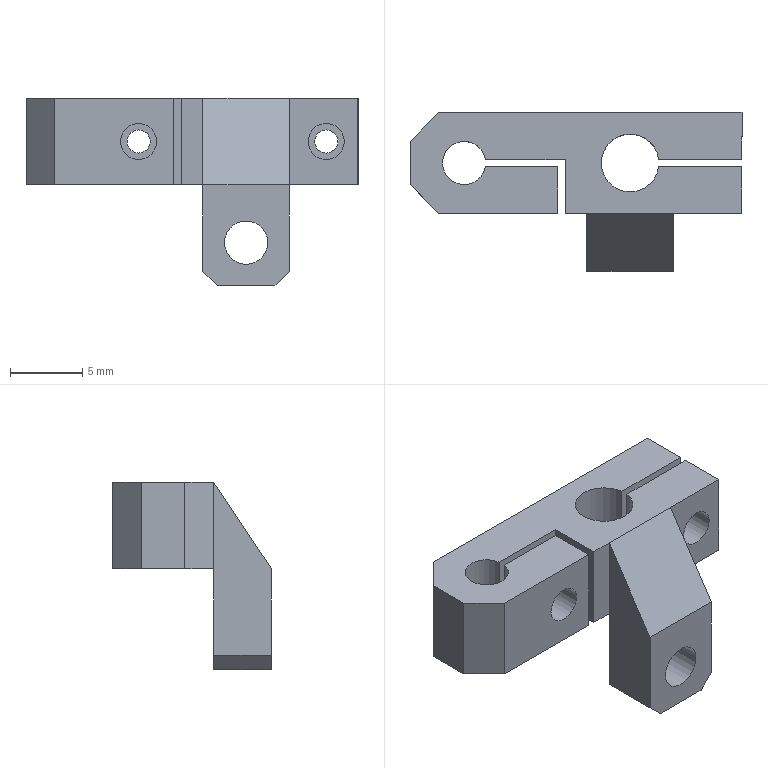Part | SolidWorks | features ICE 9, Chamfer 3, Extrusion 1, HoleWzd 1 | 1 solid | 39 faces | box 23 x 11 x 13 mm | volume 943.404 mm3 | plane 25 | cylinder 14 | commonest cylinder face diameters 1.6 x4 2.5 x4 3 x4 4 x2
STEP:
#1=CARTESIAN_POINT('',(-0.7,0.25,9.2));
#2=VERTEX_POINT('',#1);
#3=CARTESIAN_POINT('',(-0.7,0.25,10.8));
#4=VERTEX_POINT('',#3);
#5=CARTESIAN_POINT('',(-0.7,0.25,10.));
#6=DIRECTION('',(0.,1.,0.));
#7=DIRECTION('',(-1.,0.,0.));
#8=AXIS2_PLACEMENT_3D('',#5,#6,#7);
#9=CIRCLE('',#8,0.8);
#10=EDGE_CURVE('',#2,#4,#9,.T.);
#11=ORIENTED_EDGE('',*,*,#10,.F.);
#12=CARTESIAN_POINT('',(-0.7,3.5,9.2));
#13=VERTEX_POINT('',#12);
#14=CARTESIAN_POINT('',(-0.7,3.5,9.2));
#15=DIRECTION('',(0.,1.,0.));
#16=VECTOR('',#15,1000.);
#17=LINE('',#14,#16);
#18=EDGE_CURVE('',#2,#13,#17,.T.);
#19=ORIENTED_EDGE('',*,*,#18,.T.);
#20=CARTESIAN_POINT('',(-0.7,3.5,10.8));
#21=VERTEX_POINT('',#20);
#22=CARTESIAN_POINT('',(-0.7,3.5,10.));
#23=DIRECTION('',(0.,1.,0.));
#24=DIRECTION('',(0.,0.,1.));
#25=AXIS2_PLACEMENT_3D('',#22,#23,#24);
#26=CIRCLE('',#25,0.8);
#27=EDGE_CURVE('',#13,#21,#26,.T.);
#28=ORIENTED_EDGE('',*,*,#27,.T.);
#29=CARTESIAN_POINT('',(-0.7,3.5,10.8));
#30=DIRECTION('',(0.,1.,0.));
#31=VECTOR('',#30,1000.);
#32=LINE('',#29,#31);
#33=EDGE_CURVE('',#4,#21,#32,.T.);
#34=ORIENTED_EDGE('',*,*,#33,.F.);
#35=EDGE_LOOP('',(#11,#19,#28,#34));
#36=FACE_OUTER_BOUND('',#35,.T.);
#37=CARTESIAN_POINT('',(-0.7,3.5,10.));
#38=DIRECTION('',(0.,1.,0.));
#39=DIRECTION('',(0.,0.,1.));
#40=AXIS2_PLACEMENT_3D('',#37,#38,#39);
#41=CYLINDRICAL_SURFACE('',#40,0.8);
#42=ADVANCED_FACE('',(#36),#41,.F.);
#43=CARTESIAN_POINT('',(12.3,0.25,9.2));
#44=VERTEX_POINT('',#43);
#45=CARTESIAN_POINT('',(12.3,0.25,10.8));
#46=VERTEX_POINT('',#45);
#47=CARTESIAN_POINT('',(12.3,0.25,10.));
#48=DIRECTION('',(0.,1.,0.));
#49=DIRECTION('',(-1.,0.,0.));
#50=AXIS2_PLACEMENT_3D('',#47,#48,#49);
#51=CIRCLE('',#50,0.8);
#52=EDGE_CURVE('',#44,#46,#51,.T.);
#53=ORIENTED_EDGE('',*,*,#52,.F.);
#54=CARTESIAN_POINT('',(12.3,3.5,9.2));
#55=VERTEX_POINT('',#54);
#56=CARTESIAN_POINT('',(12.3,3.5,9.2));
#57=DIRECTION('',(0.,1.,0.));
#58=VECTOR('',#57,1000.);
#59=LINE('',#56,#58);
#60=EDGE_CURVE('',#44,#55,#59,.T.);
#61=ORIENTED_EDGE('',*,*,#60,.T.);
#62=CARTESIAN_POINT('',(12.3,3.5,10.8));
#63=VERTEX_POINT('',#62);
#64=CARTESIAN_POINT('',(12.3,3.5,10.));
#65=DIRECTION('',(0.,1.,0.));
#66=DIRECTION('',(0.,0.,1.));
#67=AXIS2_PLACEMENT_3D('',#64,#65,#66);
#68=CIRCLE('',#67,0.8);
#69=EDGE_CURVE('',#55,#63,#68,.T.);
#70=ORIENTED_EDGE('',*,*,#69,.T.);
#71=CARTESIAN_POINT('',(12.3,3.5,10.8));
#72=DIRECTION('',(0.,1.,0.));
#73=VECTOR('',#72,1000.);
#74=LINE('',#71,#73);
#75=EDGE_CURVE('',#46,#63,#74,.T.);
#76=ORIENTED_EDGE('',*,*,#75,.F.);
#77=EDGE_LOOP('',(#53,#61,#70,#76));
#78=FACE_OUTER_BOUND('',#77,.T.);
#79=CARTESIAN_POINT('',(12.3,3.5,10.));
#80=DIRECTION('',(0.,1.,0.));
#81=DIRECTION('',(0.,0.,1.));
#82=AXIS2_PLACEMENT_3D('',#79,#80,#81);
#83=CYLINDRICAL_SURFACE('',#82,0.8);
#84=ADVANCED_FACE('',(#78),#83,.F.);
#85=CARTESIAN_POINT('',(5.25,-3.5,3.));
#86=VERTEX_POINT('',#85);
#87=CARTESIAN_POINT('',(8.25,-3.5,3.));
#88=VERTEX_POINT('',#87);
#89=CARTESIAN_POINT('',(6.75,-3.5,3.));
#90=DIRECTION('',(0.,-1.,0.));
#91=DIRECTION('',(1.,0.,0.));
#92=AXIS2_PLACEMENT_3D('',#89,#90,#91);
#93=CIRCLE('',#92,1.5);
#94=EDGE_CURVE('',#86,#88,#93,.T.);
#95=ORIENTED_EDGE('',*,*,#94,.F.);
#96=CARTESIAN_POINT('',(5.25,-7.5,3.));
#97=VERTEX_POINT('',#96);
#98=CARTESIAN_POINT('',(5.25,0.5,3.));
#99=DIRECTION('',(0.,-1.,0.));
#100=VECTOR('',#99,1000.);
#101=LINE('',#98,#100);
#102=EDGE_CURVE('',#86,#97,#101,.T.);
#103=ORIENTED_EDGE('',*,*,#102,.T.);
#104=CARTESIAN_POINT('',(8.25,-7.5,3.));
#105=VERTEX_POINT('',#104);
#106=CARTESIAN_POINT('',(6.75,-7.5,3.));
#107=DIRECTION('',(0.,-1.,0.));
#108=DIRECTION('',(1.,0.,0.));
#109=AXIS2_PLACEMENT_3D('',#106,#107,#108);
#110=CIRCLE('',#109,1.5);
#111=EDGE_CURVE('',#97,#105,#110,.T.);
#112=ORIENTED_EDGE('',*,*,#111,.T.);
#113=CARTESIAN_POINT('',(8.25,0.5,3.));
#114=DIRECTION('',(0.,-1.,0.));
#115=VECTOR('',#114,1000.);
#116=LINE('',#113,#115);
#117=EDGE_CURVE('',#88,#105,#116,.T.);
#118=ORIENTED_EDGE('',*,*,#117,.F.);
#119=EDGE_LOOP('',(#95,#103,#112,#118));
#120=FACE_OUTER_BOUND('',#119,.T.);
#121=CARTESIAN_POINT('',(6.75,0.5,3.));
#122=DIRECTION('',(0.,-1.,0.));
#123=DIRECTION('',(1.,0.,0.));
#124=AXIS2_PLACEMENT_3D('',#121,#122,#123);
#125=CYLINDRICAL_SURFACE('',#124,1.5);
#126=ADVANCED_FACE('',(#120),#125,.F.);
#127=CARTESIAN_POINT('',(0.55,-0.25,10.));
#128=VERTEX_POINT('',#127);
#129=CARTESIAN_POINT('',(-1.95,-0.25,10.));
#130=VERTEX_POINT('',#129);
#131=CARTESIAN_POINT('',(-0.7,-0.25,10.));
#132=DIRECTION('',(0.,1.,0.));
#133=DIRECTION('',(0.,0.,-1.));
#134=AXIS2_PLACEMENT_3D('',#131,#132,#133);
#135=CIRCLE('',#134,1.25);
#136=EDGE_CURVE('',#128,#130,#135,.T.);
#137=ORIENTED_EDGE('',*,*,#136,.T.);
#138=CARTESIAN_POINT('',(-1.95,-3.5,10.));
#139=VERTEX_POINT('',#138);
#140=CARTESIAN_POINT('',(-1.95,3.286,10.));
#141=DIRECTION('',(0.,-1.,0.));
#142=VECTOR('',#141,1000.);
#143=LINE('',#140,#142);
#144=EDGE_CURVE('',#130,#139,#143,.T.);
#145=ORIENTED_EDGE('',*,*,#144,.T.);
#146=CARTESIAN_POINT('',(0.55,-3.5,10.));
#147=VERTEX_POINT('',#146);
#148=CARTESIAN_POINT('',(-0.7,-3.5,10.));
#149=DIRECTION('',(0.,-1.,0.));
#150=DIRECTION('',(1.,0.,0.));
#151=AXIS2_PLACEMENT_3D('',#148,#149,#150);
#152=CIRCLE('',#151,1.25);
#153=EDGE_CURVE('',#139,#147,#152,.T.);
#154=ORIENTED_EDGE('',*,*,#153,.T.);
#155=CARTESIAN_POINT('',(0.55,3.286,10.));
#156=DIRECTION('',(0.,-1.,0.));
#157=VECTOR('',#156,1000.);
#158=LINE('',#155,#157);
#159=EDGE_CURVE('',#128,#147,#158,.T.);
#160=ORIENTED_EDGE('',*,*,#159,.F.);
#161=EDGE_LOOP('',(#137,#145,#154,#160));
#162=FACE_OUTER_BOUND('',#161,.T.);
#163=CARTESIAN_POINT('',(-0.7,3.286,10.));
#164=DIRECTION('',(0.,-1.,0.));
#165=DIRECTION('',(1.,0.,0.));
#166=AXIS2_PLACEMENT_3D('',#163,#164,#165);
#167=CYLINDRICAL_SURFACE('',#166,1.25);
#168=ADVANCED_FACE('',(#162),#167,.F.);
#169=CARTESIAN_POINT('',(13.55,-0.25,10.));
#170=VERTEX_POINT('',#169);
#171=CARTESIAN_POINT('',(11.05,-0.25,10.));
#172=VERTEX_POINT('',#171);
#173=CARTESIAN_POINT('',(12.3,-0.25,10.));
#174=DIRECTION('',(0.,1.,0.));
#175=DIRECTION('',(0.,0.,-1.));
#176=AXIS2_PLACEMENT_3D('',#173,#174,#175);
#177=CIRCLE('',#176,1.25);
#178=EDGE_CURVE('',#170,#172,#177,.T.);
#179=ORIENTED_EDGE('',*,*,#178,.T.);
#180=CARTESIAN_POINT('',(11.05,-3.5,10.));
#181=VERTEX_POINT('',#180);
#182=CARTESIAN_POINT('',(11.05,3.286,10.));
#183=DIRECTION('',(0.,-1.,0.));
#184=VECTOR('',#183,1000.);
#185=LINE('',#182,#184);
#186=EDGE_CURVE('',#172,#181,#185,.T.);
#187=ORIENTED_EDGE('',*,*,#186,.T.);
#188=CARTESIAN_POINT('',(13.55,-3.5,10.));
#189=VERTEX_POINT('',#188);
#190=CARTESIAN_POINT('',(12.3,-3.5,10.));
#191=DIRECTION('',(0.,-1.,0.));
#192=DIRECTION('',(1.,0.,0.));
#193=AXIS2_PLACEMENT_3D('',#190,#191,#192);
#194=CIRCLE('',#193,1.25);
#195=EDGE_CURVE('',#181,#189,#194,.T.);
#196=ORIENTED_EDGE('',*,*,#195,.T.);
#197=CARTESIAN_POINT('',(13.55,3.286,10.));
#198=DIRECTION('',(0.,-1.,0.));
#199=VECTOR('',#198,1000.);
#200=LINE('',#197,#199);
#201=EDGE_CURVE('',#170,#189,#200,.T.);
#202=ORIENTED_EDGE('',*,*,#201,.F.);
#203=EDGE_LOOP('',(#179,#187,#196,#202));
#204=FACE_OUTER_BOUND('',#203,.T.);
#205=CARTESIAN_POINT('',(12.3,3.286,10.));
#206=DIRECTION('',(0.,-1.,0.));
#207=DIRECTION('',(1.,0.,0.));
#208=AXIS2_PLACEMENT_3D('',#205,#206,#207);
#209=CYLINDRICAL_SURFACE('',#208,1.25);
#210=ADVANCED_FACE('',(#204),#209,.F.);
#211=CARTESIAN_POINT('',(-3.271,0.25,13.));
#212=VERTEX_POINT('',#211);
#213=CARTESIAN_POINT('',(-6.25,0.,13.));
#214=VERTEX_POINT('',#213);
#215=CARTESIAN_POINT('',(-4.75,0.,13.));
#216=DIRECTION('',(0.,0.,1.));
#217=DIRECTION('',(1.,0.,0.));
#218=AXIS2_PLACEMENT_3D('',#215,#216,#217);
#219=CIRCLE('',#218,1.5);
#220=EDGE_CURVE('',#212,#214,#219,.T.);
#221=ORIENTED_EDGE('',*,*,#220,.T.);
#222=CARTESIAN_POINT('',(-6.25,0.,7.));
#223=VERTEX_POINT('',#222);
#224=CARTESIAN_POINT('',(-6.25,0.,13.));
#225=DIRECTION('',(0.,0.,-1.));
#226=VECTOR('',#225,1000.);
#227=LINE('',#224,#226);
#228=EDGE_CURVE('',#214,#223,#227,.T.);
#229=ORIENTED_EDGE('',*,*,#228,.T.);
#230=CARTESIAN_POINT('',(-3.271,0.25,7.));
#231=VERTEX_POINT('',#230);
#232=CARTESIAN_POINT('',(-4.75,0.,7.));
#233=DIRECTION('',(0.,0.,-1.));
#234=DIRECTION('',(-1.,0.,0.));
#235=AXIS2_PLACEMENT_3D('',#232,#233,#234);
#236=CIRCLE('',#235,1.5);
#237=EDGE_CURVE('',#223,#231,#236,.T.);
#238=ORIENTED_EDGE('',*,*,#237,.T.);
#239=CARTESIAN_POINT('',(-3.271,0.25,13.));
#240=DIRECTION('',(0.,0.,-1.));
#241=VECTOR('',#240,1000.);
#242=LINE('',#239,#241);
#243=EDGE_CURVE('',#212,#231,#242,.T.);
#244=ORIENTED_EDGE('',*,*,#243,.F.);
#245=EDGE_LOOP('',(#221,#229,#238,#244));
#246=FACE_OUTER_BOUND('',#245,.T.);
#247=CARTESIAN_POINT('',(-4.75,0.,13.));
#248=DIRECTION('',(0.,0.,-1.));
#249=DIRECTION('',(-1.,0.,0.));
#250=AXIS2_PLACEMENT_3D('',#247,#248,#249);
#251=CYLINDRICAL_SURFACE('',#250,1.5);
#252=ADVANCED_FACE('',(#246),#251,.F.);
#253=CARTESIAN_POINT('',(8.734,0.25,13.));
#254=VERTEX_POINT('',#253);
#255=CARTESIAN_POINT('',(4.75,0.,13.));
#256=VERTEX_POINT('',#255);
#257=CARTESIAN_POINT('',(6.75,0.,13.));
#258=DIRECTION('',(0.,0.,1.));
#259=DIRECTION('',(1.,0.,0.));
#260=AXIS2_PLACEMENT_3D('',#257,#258,#259);
#261=CIRCLE('',#260,2.);
#262=EDGE_CURVE('',#254,#256,#261,.T.);
#263=ORIENTED_EDGE('',*,*,#262,.T.);
#264=CARTESIAN_POINT('',(4.75,0.,7.));
#265=VERTEX_POINT('',#264);
#266=CARTESIAN_POINT('',(4.75,0.,13.));
#267=DIRECTION('',(0.,0.,-1.));
#268=VECTOR('',#267,1000.);
#269=LINE('',#266,#268);
#270=EDGE_CURVE('',#256,#265,#269,.T.);
#271=ORIENTED_EDGE('',*,*,#270,.T.);
#272=CARTESIAN_POINT('',(8.734,0.25,7.));
#273=VERTEX_POINT('',#272);
#274=CARTESIAN_POINT('',(6.75,0.,7.));
#275=DIRECTION('',(0.,0.,-1.));
#276=DIRECTION('',(-1.,0.,0.));
#277=AXIS2_PLACEMENT_3D('',#274,#275,#276);
#278=CIRCLE('',#277,2.);
#279=EDGE_CURVE('',#265,#273,#278,.T.);
#280=ORIENTED_EDGE('',*,*,#279,.T.);
#281=CARTESIAN_POINT('',(8.734,0.25,13.));
#282=DIRECTION('',(0.,0.,-1.));
#283=VECTOR('',#282,1000.);
#284=LINE('',#281,#283);
#285=EDGE_CURVE('',#254,#273,#284,.T.);
#286=ORIENTED_EDGE('',*,*,#285,.F.);
#287=EDGE_LOOP('',(#263,#271,#280,#286));
#288=FACE_OUTER_BOUND('',#287,.T.);
#289=CARTESIAN_POINT('',(6.75,0.,13.));
#290=DIRECTION('',(0.,0.,-1.));
#291=DIRECTION('',(-1.,0.,0.));
#292=AXIS2_PLACEMENT_3D('',#289,#290,#291);
#293=CYLINDRICAL_SURFACE('',#292,2.);
#294=ADVANCED_FACE('',(#288),#293,.F.);
#295=CARTESIAN_POINT('',(1.75,-3.5,13.));
#296=VERTEX_POINT('',#295);
#297=CARTESIAN_POINT('',(-6.5,-3.5,13.));
#298=VERTEX_POINT('',#297);
#299=CARTESIAN_POINT('',(-14.5,-3.5,13.));
#300=DIRECTION('',(-1.,0.,0.));
#301=VECTOR('',#300,1000.);
#302=LINE('',#299,#301);
#303=EDGE_CURVE('',#296,#298,#302,.T.);
#304=ORIENTED_EDGE('',*,*,#303,.T.);
#305=CARTESIAN_POINT('',(-6.5,-3.5,7.));
#306=VERTEX_POINT('',#305);
#307=CARTESIAN_POINT('',(-6.5,-3.5,7.));
#308=DIRECTION('',(0.,0.,-1.));
#309=VECTOR('',#308,1000.);
#310=LINE('',#307,#309);
#311=EDGE_CURVE('',#298,#306,#310,.T.);
#312=ORIENTED_EDGE('',*,*,#311,.T.);
#313=CARTESIAN_POINT('',(1.75,-3.5,7.));
#314=VERTEX_POINT('',#313);
#315=CARTESIAN_POINT('',(14.5,-3.5,7.));
#316=DIRECTION('',(-1.,0.,0.));
#317=VECTOR('',#316,1000.);
#318=LINE('',#315,#317);
#319=EDGE_CURVE('',#314,#306,#318,.T.);
#320=ORIENTED_EDGE('',*,*,#319,.F.);
#321=CARTESIAN_POINT('',(1.75,-3.5,16.));
#322=DIRECTION('',(0.,0.,-1.));
#323=VECTOR('',#322,1000.);
#324=LINE('',#321,#323);
#325=EDGE_CURVE('',#296,#314,#324,.T.);
#326=ORIENTED_EDGE('',*,*,#325,.F.);
#327=EDGE_LOOP('',(#304,#312,#320,#326));
#328=FACE_OUTER_BOUND('',#327,.T.);
#329=CARTESIAN_POINT('',(-0.7,-3.5,10.));
#330=DIRECTION('',(0.,-1.,0.));
#331=DIRECTION('',(1.,0.,0.));
#332=AXIS2_PLACEMENT_3D('',#329,#330,#331);
#333=CIRCLE('',#332,1.25);
#334=EDGE_CURVE('',#147,#139,#333,.T.);
#335=ORIENTED_EDGE('',*,*,#334,.F.);
#336=ORIENTED_EDGE('',*,*,#153,.F.);
#337=EDGE_LOOP('',(#335,#336));
#338=FACE_BOUND('',#337,.T.);
#339=CARTESIAN_POINT('',(0.,-3.5,0.));
#340=DIRECTION('',(0.,-1.,0.));
#341=DIRECTION('',(1.,0.,0.));
#342=AXIS2_PLACEMENT_3D('',#339,#340,#341);
#343=PLANE('',#342);
#344=ADVANCED_FACE('',(#328,#338),#343,.T.);
#345=CARTESIAN_POINT('',(14.5,-0.25,7.));
#346=VERTEX_POINT('',#345);
#347=CARTESIAN_POINT('',(14.5,-3.5,7.));
#348=VERTEX_POINT('',#347);
#349=CARTESIAN_POINT('',(14.5,-3.5,7.));
#350=DIRECTION('',(0.,-1.,0.));
#351=VECTOR('',#350,1000.);
#352=LINE('',#349,#351);
#353=EDGE_CURVE('',#346,#348,#352,.T.);
#354=ORIENTED_EDGE('',*,*,#353,.F.);
#355=CARTESIAN_POINT('',(14.5,-0.25,13.));
#356=VERTEX_POINT('',#355);
#357=CARTESIAN_POINT('',(14.5,-0.25,16.));
#358=DIRECTION('',(0.,0.,-1.));
#359=VECTOR('',#358,1000.);
#360=LINE('',#357,#359);
#361=EDGE_CURVE('',#356,#346,#360,.T.);
#362=ORIENTED_EDGE('',*,*,#361,.F.);
#363=CARTESIAN_POINT('',(14.5,-3.5,13.));
#364=VERTEX_POINT('',#363);
#365=CARTESIAN_POINT('',(14.5,7.5,13.));
#366=DIRECTION('',(0.,1.,0.));
#367=VECTOR('',#366,1000.);
#368=LINE('',#365,#367);
#369=EDGE_CURVE('',#364,#356,#368,.T.);
#370=ORIENTED_EDGE('',*,*,#369,.F.);
#371=CARTESIAN_POINT('',(14.5,-3.5,13.));
#372=DIRECTION('',(0.,0.,1.));
#373=VECTOR('',#372,1000.);
#374=LINE('',#371,#373);
#375=EDGE_CURVE('',#348,#364,#374,.T.);
#376=ORIENTED_EDGE('',*,*,#375,.F.);
#377=EDGE_LOOP('',(#354,#362,#370,#376));
#378=FACE_OUTER_BOUND('',#377,.T.);
#379=CARTESIAN_POINT('',(14.5,7.5,13.));
#380=DIRECTION('',(-1.,0.,0.));
#381=DIRECTION('',(0.,-1.,0.));
#382=AXIS2_PLACEMENT_3D('',#379,#380,#381);
#383=PLANE('',#382);
#384=ADVANCED_FACE('',(#378),#383,.F.);
#385=CARTESIAN_POINT('',(14.5,0.25,13.));
#386=VERTEX_POINT('',#385);
#387=CARTESIAN_POINT('',(14.5,3.5,13.));
#388=VERTEX_POINT('',#387);
#389=CARTESIAN_POINT('',(14.5,7.5,13.));
#390=DIRECTION('',(0.,1.,0.));
#391=VECTOR('',#390,1000.);
#392=LINE('',#389,#391);
#393=EDGE_CURVE('',#386,#388,#392,.T.);
#394=ORIENTED_EDGE('',*,*,#393,.F.);
#395=CARTESIAN_POINT('',(14.5,0.25,7.));
#396=VERTEX_POINT('',#395);
#397=CARTESIAN_POINT('',(14.5,0.25,16.));
#398=DIRECTION('',(0.,0.,-1.));
#399=VECTOR('',#398,1000.);
#400=LINE('',#397,#399);
#401=EDGE_CURVE('',#386,#396,#400,.T.);
#402=ORIENTED_EDGE('',*,*,#401,.T.);
#403=CARTESIAN_POINT('',(14.5,3.5,7.));
#404=VERTEX_POINT('',#403);
#405=CARTESIAN_POINT('',(14.5,-3.5,7.));
#406=DIRECTION('',(0.,-1.,0.));
#407=VECTOR('',#406,1000.);
#408=LINE('',#405,#407);
#409=EDGE_CURVE('',#404,#396,#408,.T.);
#410=ORIENTED_EDGE('',*,*,#409,.F.);
#411=CARTESIAN_POINT('',(14.5,3.5,27.));
#412=DIRECTION('',(0.,0.,-1.));
#413=VECTOR('',#412,1000.);
#414=LINE('',#411,#413);
#415=EDGE_CURVE('',#388,#404,#414,.T.);
#416=ORIENTED_EDGE('',*,*,#415,.F.);
#417=EDGE_LOOP('',(#394,#402,#410,#416));
#418=FACE_OUTER_BOUND('',#417,.T.);
#419=CARTESIAN_POINT('',(14.5,7.5,13.));
#420=DIRECTION('',(-1.,0.,0.));
#421=DIRECTION('',(0.,-1.,0.));
#422=AXIS2_PLACEMENT_3D('',#419,#420,#421);
#423=PLANE('',#422);
#424=ADVANCED_FACE('',(#418),#423,.F.);
#425=ORIENTED_EDGE('',*,*,#270,.F.);
#426=CARTESIAN_POINT('',(8.734,-0.25,13.));
#427=VERTEX_POINT('',#426);
#428=CARTESIAN_POINT('',(6.75,0.,13.));
#429=DIRECTION('',(0.,0.,1.));
#430=DIRECTION('',(1.,0.,0.));
#431=AXIS2_PLACEMENT_3D('',#428,#429,#430);
#432=CIRCLE('',#431,2.);
#433=EDGE_CURVE('',#256,#427,#432,.T.);
#434=ORIENTED_EDGE('',*,*,#433,.T.);
#435=CARTESIAN_POINT('',(8.734,-0.25,7.));
#436=VERTEX_POINT('',#435);
#437=CARTESIAN_POINT('',(8.734,-0.25,13.));
#438=DIRECTION('',(0.,0.,1.));
#439=VECTOR('',#438,1000.);
#440=LINE('',#437,#439);
#441=EDGE_CURVE('',#436,#427,#440,.T.);
#442=ORIENTED_EDGE('',*,*,#441,.F.);
#443=CARTESIAN_POINT('',(6.75,0.,7.));
#444=DIRECTION('',(0.,0.,-1.));
#445=DIRECTION('',(-1.,0.,0.));
#446=AXIS2_PLACEMENT_3D('',#443,#444,#445);
#447=CIRCLE('',#446,2.);
#448=EDGE_CURVE('',#436,#265,#447,.T.);
#449=ORIENTED_EDGE('',*,*,#448,.T.);
#450=EDGE_LOOP('',(#425,#434,#442,#449));
#451=FACE_OUTER_BOUND('',#450,.T.);
#452=CARTESIAN_POINT('',(6.75,0.,13.));
#453=DIRECTION('',(0.,0.,-1.));
#454=DIRECTION('',(-1.,0.,0.));
#455=AXIS2_PLACEMENT_3D('',#452,#453,#454);
#456=CYLINDRICAL_SURFACE('',#455,2.);
#457=ADVANCED_FACE('',(#451),#456,.F.);
#458=ORIENTED_EDGE('',*,*,#228,.F.);
#459=CARTESIAN_POINT('',(-3.271,-0.25,13.));
#460=VERTEX_POINT('',#459);
#461=CARTESIAN_POINT('',(-4.75,0.,13.));
#462=DIRECTION('',(0.,0.,1.));
#463=DIRECTION('',(1.,0.,0.));
#464=AXIS2_PLACEMENT_3D('',#461,#462,#463);
#465=CIRCLE('',#464,1.5);
#466=EDGE_CURVE('',#214,#460,#465,.T.);
#467=ORIENTED_EDGE('',*,*,#466,.T.);
#468=CARTESIAN_POINT('',(-3.271,-0.25,7.));
#469=VERTEX_POINT('',#468);
#470=CARTESIAN_POINT('',(-3.271,-0.25,13.));
#471=DIRECTION('',(0.,0.,1.));
#472=VECTOR('',#471,1000.);
#473=LINE('',#470,#472);
#474=EDGE_CURVE('',#469,#460,#473,.T.);
#475=ORIENTED_EDGE('',*,*,#474,.F.);
#476=CARTESIAN_POINT('',(-4.75,0.,7.));
#477=DIRECTION('',(0.,0.,-1.));
#478=DIRECTION('',(-1.,0.,0.));
#479=AXIS2_PLACEMENT_3D('',#476,#477,#478);
#480=CIRCLE('',#479,1.5);
#481=EDGE_CURVE('',#469,#223,#480,.T.);
#482=ORIENTED_EDGE('',*,*,#481,.T.);
#483=EDGE_LOOP('',(#458,#467,#475,#482));
#484=FACE_OUTER_BOUND('',#483,.T.);
#485=CARTESIAN_POINT('',(-4.75,0.,13.));
#486=DIRECTION('',(0.,0.,-1.));
#487=DIRECTION('',(-1.,0.,0.));
#488=AXIS2_PLACEMENT_3D('',#485,#486,#487);
#489=CYLINDRICAL_SURFACE('',#488,1.5);
#490=ADVANCED_FACE('',(#484),#489,.F.);
#491=CARTESIAN_POINT('',(12.3,-3.5,10.));
#492=DIRECTION('',(0.,-1.,0.));
#493=DIRECTION('',(1.,0.,0.));
#494=AXIS2_PLACEMENT_3D('',#491,#492,#493);
#495=CIRCLE('',#494,1.25);
#496=EDGE_CURVE('',#189,#181,#495,.T.);
#497=ORIENTED_EDGE('',*,*,#496,.F.);
#498=ORIENTED_EDGE('',*,*,#195,.F.);
#499=EDGE_LOOP('',(#497,#498));
#500=FACE_BOUND('',#499,.T.);
#501=CARTESIAN_POINT('',(9.75,-3.5,7.));
#502=VERTEX_POINT('',#501);
#503=CARTESIAN_POINT('',(14.5,-3.5,7.));
#504=DIRECTION('',(-1.,0.,0.));
#505=VECTOR('',#504,1000.);
#506=LINE('',#503,#505);
#507=EDGE_CURVE('',#348,#502,#506,.T.);
#508=ORIENTED_EDGE('',*,*,#507,.F.);
#509=ORIENTED_EDGE('',*,*,#375,.T.);
#510=CARTESIAN_POINT('',(9.75,-3.5,13.));
#511=VERTEX_POINT('',#510);
#512=CARTESIAN_POINT('',(14.5,-3.5,13.));
#513=DIRECTION('',(-1.,0.,0.));
#514=VECTOR('',#513,1000.);
#515=LINE('',#512,#514);
#516=EDGE_CURVE('',#364,#511,#515,.T.);
#517=ORIENTED_EDGE('',*,*,#516,.T.);
#518=CARTESIAN_POINT('',(9.75,-3.5,13.));
#519=DIRECTION('',(0.,0.,-1.));
#520=VECTOR('',#519,1000.);
#521=LINE('',#518,#520);
#522=EDGE_CURVE('',#511,#502,#521,.T.);
#523=ORIENTED_EDGE('',*,*,#522,.T.);
#524=EDGE_LOOP('',(#508,#509,#517,#523));
#525=FACE_OUTER_BOUND('',#524,.T.);
#526=CARTESIAN_POINT('',(0.,-3.5,0.));
#527=DIRECTION('',(0.,1.,0.));
#528=DIRECTION('',(0.,0.,1.));
#529=AXIS2_PLACEMENT_3D('',#526,#527,#528);
#530=PLANE('',#529);
#531=ADVANCED_FACE('',(#500,#525),#530,.F.);
#532=CARTESIAN_POINT('',(2.25,-3.5,13.));
#533=VERTEX_POINT('',#532);
#534=CARTESIAN_POINT('',(2.25,-3.5,7.));
#535=VERTEX_POINT('',#534);
#536=CARTESIAN_POINT('',(2.25,-3.5,16.));
#537=DIRECTION('',(0.,0.,-1.));
#538=VECTOR('',#537,1000.);
#539=LINE('',#536,#538);
#540=EDGE_CURVE('',#533,#535,#539,.T.);
#541=ORIENTED_EDGE('',*,*,#540,.T.);
#542=CARTESIAN_POINT('',(3.75,-3.5,7.));
#543=VERTEX_POINT('',#542);
#544=CARTESIAN_POINT('',(14.5,-3.5,7.));
#545=DIRECTION('',(-1.,0.,0.));
#546=VECTOR('',#545,1000.);
#547=LINE('',#544,#546);
#548=EDGE_CURVE('',#543,#535,#547,.T.);
#549=ORIENTED_EDGE('',*,*,#548,.F.);
#550=CARTESIAN_POINT('',(3.75,-3.5,13.));
#551=VERTEX_POINT('',#550);
#552=CARTESIAN_POINT('',(3.75,-3.5,13.));
#553=DIRECTION('',(0.,0.,1.));
#554=VECTOR('',#553,1000.);
#555=LINE('',#552,#554);
#556=EDGE_CURVE('',#543,#551,#555,.T.);
#557=ORIENTED_EDGE('',*,*,#556,.T.);
#558=CARTESIAN_POINT('',(-14.5,-3.5,13.));
#559=DIRECTION('',(-1.,0.,0.));
#560=VECTOR('',#559,1000.);
#561=LINE('',#558,#560);
#562=EDGE_CURVE('',#551,#533,#561,.T.);
#563=ORIENTED_EDGE('',*,*,#562,.T.);
#564=EDGE_LOOP('',(#541,#549,#557,#563));
#565=FACE_OUTER_BOUND('',#564,.T.);
#566=CARTESIAN_POINT('',(0.,-3.5,0.));
#567=DIRECTION('',(0.,-1.,0.));
#568=DIRECTION('',(1.,0.,0.));
#569=AXIS2_PLACEMENT_3D('',#566,#567,#568);
#570=PLANE('',#569);
#571=ADVANCED_FACE('',(#565),#570,.T.);
#572=CARTESIAN_POINT('',(-0.7,3.5,10.));
#573=DIRECTION('',(0.,1.,0.));
#574=DIRECTION('',(0.,0.,1.));
#575=AXIS2_PLACEMENT_3D('',#572,#573,#574);
#576=CIRCLE('',#575,0.8);
#577=EDGE_CURVE('',#21,#13,#576,.T.);
#578=ORIENTED_EDGE('',*,*,#577,.F.);
#579=ORIENTED_EDGE('',*,*,#27,.F.);
#580=EDGE_LOOP('',(#578,#579));
#581=FACE_BOUND('',#580,.T.);
#582=CARTESIAN_POINT('',(12.3,3.5,10.));
#583=DIRECTION('',(0.,1.,0.));
#584=DIRECTION('',(0.,0.,1.));
#585=AXIS2_PLACEMENT_3D('',#582,#583,#584);
#586=CIRCLE('',#585,0.8);
#587=EDGE_CURVE('',#63,#55,#586,.T.);
#588=ORIENTED_EDGE('',*,*,#587,.F.);
#589=ORIENTED_EDGE('',*,*,#69,.F.);
#590=EDGE_LOOP('',(#588,#589));
#591=FACE_BOUND('',#590,.T.);
#592=CARTESIAN_POINT('',(-6.5,3.5,7.));
#593=VERTEX_POINT('',#592);
#594=CARTESIAN_POINT('',(14.5,3.5,7.));
#595=DIRECTION('',(1.,0.,0.));
#596=VECTOR('',#595,1000.);
#597=LINE('',#594,#596);
#598=EDGE_CURVE('',#593,#404,#597,.T.);
#599=ORIENTED_EDGE('',*,*,#598,.F.);
#600=CARTESIAN_POINT('',(-6.5,3.5,13.));
#601=VERTEX_POINT('',#600);
#602=CARTESIAN_POINT('',(-6.5,3.5,27.));
#603=DIRECTION('',(0.,0.,1.));
#604=VECTOR('',#603,1000.);
#605=LINE('',#602,#604);
#606=EDGE_CURVE('',#593,#601,#605,.T.);
#607=ORIENTED_EDGE('',*,*,#606,.T.);
#608=CARTESIAN_POINT('',(0.,3.5,13.));
#609=DIRECTION('',(1.,0.,0.));
#610=VECTOR('',#609,1000.);
#611=LINE('',#608,#610);
#612=EDGE_CURVE('',#601,#388,#611,.T.);
#613=ORIENTED_EDGE('',*,*,#612,.T.);
#614=ORIENTED_EDGE('',*,*,#415,.T.);
#615=EDGE_LOOP('',(#599,#607,#613,#614));
#616=FACE_OUTER_BOUND('',#615,.T.);
#617=CARTESIAN_POINT('',(14.5,3.5,27.));
#618=DIRECTION('',(0.,-1.,0.));
#619=DIRECTION('',(0.,0.,-1.));
#620=AXIS2_PLACEMENT_3D('',#617,#618,#619);
#621=PLANE('',#620);
#622=ADVANCED_FACE('',(#581,#591,#616),#621,.F.);
#623=ORIENTED_EDGE('',*,*,#612,.F.);
#624=CARTESIAN_POINT('',(-8.5,1.5,13.));
#625=VERTEX_POINT('',#624);
#626=CARTESIAN_POINT('',(-5.,5.,13.));
#627=DIRECTION('',(-0.7071,-0.7071,0.));
#628=VECTOR('',#627,1000.);
#629=LINE('',#626,#628);
#630=EDGE_CURVE('',#601,#625,#629,.T.);
#631=ORIENTED_EDGE('',*,*,#630,.T.);
#632=CARTESIAN_POINT('',(-8.5,-1.5,13.));
#633=VERTEX_POINT('',#632);
#634=CARTESIAN_POINT('',(-8.5,0.,13.));
#635=DIRECTION('',(0.,1.,0.));
#636=VECTOR('',#635,1000.);
#637=LINE('',#634,#636);
#638=EDGE_CURVE('',#633,#625,#637,.T.);
#639=ORIENTED_EDGE('',*,*,#638,.F.);
#640=CARTESIAN_POINT('',(-5.,-5.,13.));
#641=DIRECTION('',(0.7071,-0.7071,0.));
#642=VECTOR('',#641,1000.);
#643=LINE('',#640,#642);
#644=EDGE_CURVE('',#633,#298,#643,.T.);
#645=ORIENTED_EDGE('',*,*,#644,.T.);
#646=ORIENTED_EDGE('',*,*,#303,.F.);
#647=CARTESIAN_POINT('',(1.75,-0.25,13.));
#648=VERTEX_POINT('',#647);
#649=CARTESIAN_POINT('',(1.75,0.,13.));
#650=DIRECTION('',(0.,-1.,0.));
#651=VECTOR('',#650,1000.);
#652=LINE('',#649,#651);
#653=EDGE_CURVE('',#648,#296,#652,.T.);
#654=ORIENTED_EDGE('',*,*,#653,.F.);
#655=CARTESIAN_POINT('',(0.,-0.25,13.));
#656=DIRECTION('',(1.,0.,0.));
#657=VECTOR('',#656,1000.);
#658=LINE('',#655,#657);
#659=EDGE_CURVE('',#460,#648,#658,.T.);
#660=ORIENTED_EDGE('',*,*,#659,.F.);
#661=ORIENTED_EDGE('',*,*,#466,.F.);
#662=ORIENTED_EDGE('',*,*,#220,.F.);
#663=CARTESIAN_POINT('',(2.25,0.25,13.));
#664=VERTEX_POINT('',#663);
#665=CARTESIAN_POINT('',(0.,0.25,13.));
#666=DIRECTION('',(-1.,0.,0.));
#667=VECTOR('',#666,1000.);
#668=LINE('',#665,#667);
#669=EDGE_CURVE('',#664,#212,#668,.T.);
#670=ORIENTED_EDGE('',*,*,#669,.F.);
#671=CARTESIAN_POINT('',(2.25,0.,13.));
#672=DIRECTION('',(0.,1.,0.));
#673=VECTOR('',#672,1000.);
#674=LINE('',#671,#673);
#675=EDGE_CURVE('',#533,#664,#674,.T.);
#676=ORIENTED_EDGE('',*,*,#675,.F.);
#677=ORIENTED_EDGE('',*,*,#562,.F.);
#678=CARTESIAN_POINT('',(9.75,-3.5,13.));
#679=DIRECTION('',(1.,0.,0.));
#680=VECTOR('',#679,1000.);
#681=LINE('',#678,#680);
#682=EDGE_CURVE('',#551,#511,#681,.T.);
#683=ORIENTED_EDGE('',*,*,#682,.T.);
#684=ORIENTED_EDGE('',*,*,#516,.F.);
#685=ORIENTED_EDGE('',*,*,#369,.T.);
#686=CARTESIAN_POINT('',(0.,-0.25,13.));
#687=DIRECTION('',(1.,0.,0.));
#688=VECTOR('',#687,1000.);
#689=LINE('',#686,#688);
#690=EDGE_CURVE('',#427,#356,#689,.T.);
#691=ORIENTED_EDGE('',*,*,#690,.F.);
#692=ORIENTED_EDGE('',*,*,#433,.F.);
#693=ORIENTED_EDGE('',*,*,#262,.F.);
#694=CARTESIAN_POINT('',(0.,0.25,13.));
#695=DIRECTION('',(-1.,0.,0.));
#696=VECTOR('',#695,1000.);
#697=LINE('',#694,#696);
#698=EDGE_CURVE('',#386,#254,#697,.T.);
#699=ORIENTED_EDGE('',*,*,#698,.F.);
#700=ORIENTED_EDGE('',*,*,#393,.T.);
#701=EDGE_LOOP('',(#623,#631,#639,#645,#646,#654,#660,#661,#662,#670,#676,#677,#683,#684,#685,#691,#692,#693,#699,#700));
#702=FACE_OUTER_BOUND('',#701,.T.);
#703=CARTESIAN_POINT('',(0.,0.,13.));
#704=DIRECTION('',(0.,0.,1.));
#705=DIRECTION('',(1.,0.,0.));
#706=AXIS2_PLACEMENT_3D('',#703,#704,#705);
#707=PLANE('',#706);
#708=ADVANCED_FACE('',(#702),#707,.T.);
#709=CARTESIAN_POINT('',(8.75,-3.5,0.));
#710=VERTEX_POINT('',#709);
#711=CARTESIAN_POINT('',(4.75,-3.5,0.));
#712=VERTEX_POINT('',#711);
#713=CARTESIAN_POINT('',(14.5,-3.5,0.));
#714=DIRECTION('',(-1.,0.,0.));
#715=VECTOR('',#714,1000.);
#716=LINE('',#713,#715);
#717=EDGE_CURVE('',#710,#712,#716,.T.);
#718=ORIENTED_EDGE('',*,*,#717,.F.);
#719=CARTESIAN_POINT('',(8.75,-7.5,0.));
#720=VERTEX_POINT('',#719);
#721=CARTESIAN_POINT('',(8.75,0.,0.));
#722=DIRECTION('',(0.,-1.,0.));
#723=VECTOR('',#722,1000.);
#724=LINE('',#721,#723);
#725=EDGE_CURVE('',#710,#720,#724,.T.);
#726=ORIENTED_EDGE('',*,*,#725,.T.);
#727=CARTESIAN_POINT('',(4.75,-7.5,0.));
#728=VERTEX_POINT('',#727);
#729=CARTESIAN_POINT('',(-14.5,-7.5,0.));
#730=DIRECTION('',(1.,0.,0.));
#731=VECTOR('',#730,1000.);
#732=LINE('',#729,#731);
#733=EDGE_CURVE('',#728,#720,#732,.T.);
#734=ORIENTED_EDGE('',*,*,#733,.F.);
#735=CARTESIAN_POINT('',(4.75,0.,0.));
#736=DIRECTION('',(0.,1.,0.));
#737=VECTOR('',#736,1000.);
#738=LINE('',#735,#737);
#739=EDGE_CURVE('',#728,#712,#738,.T.);
#740=ORIENTED_EDGE('',*,*,#739,.T.);
#741=EDGE_LOOP('',(#718,#726,#734,#740));
#742=FACE_OUTER_BOUND('',#741,.T.);
#743=CARTESIAN_POINT('',(0.,0.,0.));
#744=DIRECTION('',(0.,0.,1.));
#745=DIRECTION('',(1.,0.,0.));
#746=AXIS2_PLACEMENT_3D('',#743,#744,#745);
#747=PLANE('',#746);
#748=ADVANCED_FACE('',(#742),#747,.F.);
#749=CARTESIAN_POINT('',(6.75,-7.5,3.));
#750=DIRECTION('',(0.,-1.,0.));
#751=DIRECTION('',(1.,0.,0.));
#752=AXIS2_PLACEMENT_3D('',#749,#750,#751);
#753=CIRCLE('',#752,1.5);
#754=EDGE_CURVE('',#105,#97,#753,.T.);
#755=ORIENTED_EDGE('',*,*,#754,.F.);
#756=ORIENTED_EDGE('',*,*,#111,.F.);
#757=EDGE_LOOP('',(#755,#756));
#758=FACE_BOUND('',#757,.T.);
#759=ORIENTED_EDGE('',*,*,#733,.T.);
#760=CARTESIAN_POINT('',(9.75,-7.5,1.));
#761=VERTEX_POINT('',#760);
#762=CARTESIAN_POINT('',(8.75,-7.5,0.));
#763=DIRECTION('',(0.7071,0.,0.7071));
#764=VECTOR('',#763,1000.);
#765=LINE('',#762,#764);
#766=EDGE_CURVE('',#720,#761,#765,.T.);
#767=ORIENTED_EDGE('',*,*,#766,.T.);
#768=CARTESIAN_POINT('',(9.75,-7.5,7.));
#769=VERTEX_POINT('',#768);
#770=CARTESIAN_POINT('',(9.75,-7.5,13.));
#771=DIRECTION('',(0.,0.,-1.));
#772=VECTOR('',#771,1000.);
#773=LINE('',#770,#772);
#774=EDGE_CURVE('',#769,#761,#773,.T.);
#775=ORIENTED_EDGE('',*,*,#774,.F.);
#776=CARTESIAN_POINT('',(3.75,-7.5,7.));
#777=VERTEX_POINT('',#776);
#778=CARTESIAN_POINT('',(3.75,-7.5,7.));
#779=DIRECTION('',(-1.,0.,0.));
#780=VECTOR('',#779,1000.);
#781=LINE('',#778,#780);
#782=EDGE_CURVE('',#769,#777,#781,.T.);
#783=ORIENTED_EDGE('',*,*,#782,.T.);
#784=CARTESIAN_POINT('',(3.75,-7.5,1.));
#785=VERTEX_POINT('',#784);
#786=CARTESIAN_POINT('',(3.75,-7.5,13.));
#787=DIRECTION('',(0.,0.,1.));
#788=VECTOR('',#787,1000.);
#789=LINE('',#786,#788);
#790=EDGE_CURVE('',#785,#777,#789,.T.);
#791=ORIENTED_EDGE('',*,*,#790,.F.);
#792=CARTESIAN_POINT('',(3.75,-7.5,1.));
#793=DIRECTION('',(0.7071,0.,-0.7071));
#794=VECTOR('',#793,1000.);
#795=LINE('',#792,#794);
#796=EDGE_CURVE('',#785,#728,#795,.T.);
#797=ORIENTED_EDGE('',*,*,#796,.T.);
#798=EDGE_LOOP('',(#759,#767,#775,#783,#791,#797));
#799=FACE_OUTER_BOUND('',#798,.T.);
#800=CARTESIAN_POINT('',(-14.5,-7.5,13.));
#801=DIRECTION('',(0.,1.,0.));
#802=DIRECTION('',(-1.,0.,0.));
#803=AXIS2_PLACEMENT_3D('',#800,#801,#802);
#804=PLANE('',#803);
#805=ADVANCED_FACE('',(#758,#799),#804,.F.);
#806=ORIENTED_EDGE('',*,*,#774,.T.);
#807=CARTESIAN_POINT('',(9.75,-3.5,1.));
#808=VERTEX_POINT('',#807);
#809=CARTESIAN_POINT('',(9.75,-3.5,1.));
#810=DIRECTION('',(0.,1.,0.));
#811=VECTOR('',#810,1000.);
#812=LINE('',#809,#811);
#813=EDGE_CURVE('',#761,#808,#812,.T.);
#814=ORIENTED_EDGE('',*,*,#813,.T.);
#815=CARTESIAN_POINT('',(9.75,-3.5,13.));
#816=DIRECTION('',(0.,0.,1.));
#817=VECTOR('',#816,1000.);
#818=LINE('',#815,#817);
#819=EDGE_CURVE('',#808,#502,#818,.T.);
#820=ORIENTED_EDGE('',*,*,#819,.T.);
#821=ORIENTED_EDGE('',*,*,#522,.F.);
#822=CARTESIAN_POINT('',(9.75,-3.5,13.));
#823=DIRECTION('',(0.,-0.5547,-0.8321));
#824=VECTOR('',#823,1000.);
#825=LINE('',#822,#824);
#826=EDGE_CURVE('',#511,#769,#825,.T.);
#827=ORIENTED_EDGE('',*,*,#826,.T.);
#828=EDGE_LOOP('',(#806,#814,#820,#821,#827));
#829=FACE_OUTER_BOUND('',#828,.T.);
#830=CARTESIAN_POINT('',(9.75,-3.5,13.));
#831=DIRECTION('',(-1.,0.,0.));
#832=DIRECTION('',(0.,-1.,0.));
#833=AXIS2_PLACEMENT_3D('',#830,#831,#832);
#834=PLANE('',#833);
#835=ADVANCED_FACE('',(#829),#834,.F.);
#836=CARTESIAN_POINT('',(3.75,-3.5,1.));
#837=VERTEX_POINT('',#836);
#838=CARTESIAN_POINT('',(3.75,-3.5,13.));
#839=DIRECTION('',(0.,0.,1.));
#840=VECTOR('',#839,1000.);
#841=LINE('',#838,#840);
#842=EDGE_CURVE('',#837,#543,#841,.T.);
#843=ORIENTED_EDGE('',*,*,#842,.F.);
#844=CARTESIAN_POINT('',(3.75,-3.5,1.));
#845=DIRECTION('',(0.,-1.,0.));
#846=VECTOR('',#845,1000.);
#847=LINE('',#844,#846);
#848=EDGE_CURVE('',#837,#785,#847,.T.);
#849=ORIENTED_EDGE('',*,*,#848,.T.);
#850=ORIENTED_EDGE('',*,*,#790,.T.);
#851=CARTESIAN_POINT('',(3.75,-3.5,13.));
#852=DIRECTION('',(0.,0.5547,0.8321));
#853=VECTOR('',#852,1000.);
#854=LINE('',#851,#853);
#855=EDGE_CURVE('',#777,#551,#854,.T.);
#856=ORIENTED_EDGE('',*,*,#855,.T.);
#857=ORIENTED_EDGE('',*,*,#556,.F.);
#858=EDGE_LOOP('',(#843,#849,#850,#856,#857));
#859=FACE_OUTER_BOUND('',#858,.T.);
#860=CARTESIAN_POINT('',(3.75,-3.5,13.));
#861=DIRECTION('',(1.,0.,0.));
#862=DIRECTION('',(0.,1.,0.));
#863=AXIS2_PLACEMENT_3D('',#860,#861,#862);
#864=PLANE('',#863);
#865=ADVANCED_FACE('',(#859),#864,.F.);
#866=CARTESIAN_POINT('',(6.75,-3.5,3.));
#867=DIRECTION('',(0.,-1.,0.));
#868=DIRECTION('',(1.,0.,0.));
#869=AXIS2_PLACEMENT_3D('',#866,#867,#868);
#870=CIRCLE('',#869,1.5);
#871=EDGE_CURVE('',#88,#86,#870,.T.);
#872=ORIENTED_EDGE('',*,*,#871,.T.);
#873=ORIENTED_EDGE('',*,*,#94,.T.);
#874=EDGE_LOOP('',(#872,#873));
#875=FACE_BOUND('',#874,.T.);
#876=ORIENTED_EDGE('',*,*,#819,.F.);
#877=CARTESIAN_POINT('',(8.75,-3.5,0.));
#878=DIRECTION('',(-0.7071,0.,-0.7071));
#879=VECTOR('',#878,1000.);
#880=LINE('',#877,#879);
#881=EDGE_CURVE('',#808,#710,#880,.T.);
#882=ORIENTED_EDGE('',*,*,#881,.T.);
#883=ORIENTED_EDGE('',*,*,#717,.T.);
#884=CARTESIAN_POINT('',(3.75,-3.5,1.));
#885=DIRECTION('',(-0.7071,0.,0.7071));
#886=VECTOR('',#885,1000.);
#887=LINE('',#884,#886);
#888=EDGE_CURVE('',#712,#837,#887,.T.);
#889=ORIENTED_EDGE('',*,*,#888,.T.);
#890=ORIENTED_EDGE('',*,*,#842,.T.);
#891=CARTESIAN_POINT('',(14.5,-3.5,7.));
#892=DIRECTION('',(-1.,0.,0.));
#893=VECTOR('',#892,1000.);
#894=LINE('',#891,#893);
#895=EDGE_CURVE('',#502,#543,#894,.T.);
#896=ORIENTED_EDGE('',*,*,#895,.F.);
#897=EDGE_LOOP('',(#876,#882,#883,#889,#890,#896));
#898=FACE_OUTER_BOUND('',#897,.T.);
#899=CARTESIAN_POINT('',(14.5,-3.5,7.));
#900=DIRECTION('',(0.,-1.,0.));
#901=DIRECTION('',(1.,0.,0.));
#902=AXIS2_PLACEMENT_3D('',#899,#900,#901);
#903=PLANE('',#902);
#904=ADVANCED_FACE('',(#875,#898),#903,.F.);
#905=CARTESIAN_POINT('',(-8.5,1.5,7.));
#906=VERTEX_POINT('',#905);
#907=CARTESIAN_POINT('',(-8.5,-1.5,7.));
#908=VERTEX_POINT('',#907);
#909=CARTESIAN_POINT('',(-8.5,3.5,7.));
#910=DIRECTION('',(0.,-1.,0.));
#911=VECTOR('',#910,1000.);
#912=LINE('',#909,#911);
#913=EDGE_CURVE('',#906,#908,#912,.T.);
#914=ORIENTED_EDGE('',*,*,#913,.F.);
#915=CARTESIAN_POINT('',(-5.,5.,7.));
#916=DIRECTION('',(0.7071,0.7071,0.));
#917=VECTOR('',#916,1000.);
#918=LINE('',#915,#917);
#919=EDGE_CURVE('',#906,#593,#918,.T.);
#920=ORIENTED_EDGE('',*,*,#919,.T.);
#921=ORIENTED_EDGE('',*,*,#598,.T.);
#922=ORIENTED_EDGE('',*,*,#409,.T.);
#923=CARTESIAN_POINT('',(0.,0.25,7.));
#924=DIRECTION('',(1.,0.,0.));
#925=VECTOR('',#924,1000.);
#926=LINE('',#923,#925);
#927=EDGE_CURVE('',#273,#396,#926,.T.);
#928=ORIENTED_EDGE('',*,*,#927,.F.);
#929=ORIENTED_EDGE('',*,*,#279,.F.);
#930=ORIENTED_EDGE('',*,*,#448,.F.);
#931=CARTESIAN_POINT('',(8.,-0.25,7.));
#932=DIRECTION('',(-1.,0.,0.));
#933=VECTOR('',#932,1000.);
#934=LINE('',#931,#933);
#935=EDGE_CURVE('',#346,#436,#934,.T.);
#936=ORIENTED_EDGE('',*,*,#935,.F.);
#937=ORIENTED_EDGE('',*,*,#353,.T.);
#938=ORIENTED_EDGE('',*,*,#507,.T.);
#939=ORIENTED_EDGE('',*,*,#895,.T.);
#940=ORIENTED_EDGE('',*,*,#548,.T.);
#941=CARTESIAN_POINT('',(2.25,0.25,7.));
#942=VERTEX_POINT('',#941);
#943=CARTESIAN_POINT('',(2.25,0.25,7.));
#944=DIRECTION('',(0.,-1.,0.));
#945=VECTOR('',#944,1000.);
#946=LINE('',#943,#945);
#947=EDGE_CURVE('',#942,#535,#946,.T.);
#948=ORIENTED_EDGE('',*,*,#947,.F.);
#949=CARTESIAN_POINT('',(0.,0.25,7.));
#950=DIRECTION('',(1.,0.,0.));
#951=VECTOR('',#950,1000.);
#952=LINE('',#949,#951);
#953=EDGE_CURVE('',#231,#942,#952,.T.);
#954=ORIENTED_EDGE('',*,*,#953,.F.);
#955=ORIENTED_EDGE('',*,*,#237,.F.);
#956=ORIENTED_EDGE('',*,*,#481,.F.);
#957=CARTESIAN_POINT('',(1.75,-0.25,7.));
#958=VERTEX_POINT('',#957);
#959=CARTESIAN_POINT('',(1.75,-0.25,7.));
#960=DIRECTION('',(-1.,0.,0.));
#961=VECTOR('',#960,1000.);
#962=LINE('',#959,#961);
#963=EDGE_CURVE('',#958,#469,#962,.T.);
#964=ORIENTED_EDGE('',*,*,#963,.F.);
#965=CARTESIAN_POINT('',(1.75,-3.5,7.));
#966=DIRECTION('',(0.,1.,0.));
#967=VECTOR('',#966,1000.);
#968=LINE('',#965,#967);
#969=EDGE_CURVE('',#314,#958,#968,.T.);
#970=ORIENTED_EDGE('',*,*,#969,.F.);
#971=ORIENTED_EDGE('',*,*,#319,.T.);
#972=CARTESIAN_POINT('',(-5.,-5.,7.));
#973=DIRECTION('',(-0.7071,0.7071,0.));
#974=VECTOR('',#973,1000.);
#975=LINE('',#972,#974);
#976=EDGE_CURVE('',#306,#908,#975,.T.);
#977=ORIENTED_EDGE('',*,*,#976,.T.);
#978=EDGE_LOOP('',(#914,#920,#921,#922,#928,#929,#930,#936,#937,#938,#939,#940,#948,#954,#955,#956,#964,#970,#971,#977));
#979=FACE_OUTER_BOUND('',#978,.T.);
#980=CARTESIAN_POINT('',(0.,0.,7.));
#981=DIRECTION('',(0.,0.,-1.));
#982=DIRECTION('',(-1.,0.,0.));
#983=AXIS2_PLACEMENT_3D('',#980,#981,#982);
#984=PLANE('',#983);
#985=ADVANCED_FACE('',(#979),#984,.T.);
#986=ORIENTED_EDGE('',*,*,#855,.F.);
#987=ORIENTED_EDGE('',*,*,#782,.F.);
#988=ORIENTED_EDGE('',*,*,#826,.F.);
#989=ORIENTED_EDGE('',*,*,#682,.F.);
#990=EDGE_LOOP('',(#986,#987,#988,#989));
#991=FACE_OUTER_BOUND('',#990,.T.);
#992=CARTESIAN_POINT('',(0.,-3.5,13.));
#993=DIRECTION('',(0.,-0.8321,0.5547));
#994=DIRECTION('',(-1.,0.,0.));
#995=AXIS2_PLACEMENT_3D('',#992,#993,#994);
#996=PLANE('',#995);
#997=ADVANCED_FACE('',(#991),#996,.T.);
#998=CARTESIAN_POINT('',(12.3,0.25,10.));
#999=DIRECTION('',(0.,1.,0.));
#1000=DIRECTION('',(-1.,0.,0.));
#1001=AXIS2_PLACEMENT_3D('',#998,#999,#1000);
#1002=CIRCLE('',#1001,0.8);
#1003=EDGE_CURVE('',#46,#44,#1002,.T.);
#1004=ORIENTED_EDGE('',*,*,#1003,.T.);
#1005=ORIENTED_EDGE('',*,*,#52,.T.);
#1006=EDGE_LOOP('',(#1004,#1005));
#1007=FACE_BOUND('',#1006,.T.);
#1008=ORIENTED_EDGE('',*,*,#285,.T.);
#1009=ORIENTED_EDGE('',*,*,#927,.T.);
#1010=ORIENTED_EDGE('',*,*,#401,.F.);
#1011=ORIENTED_EDGE('',*,*,#698,.T.);
#1012=EDGE_LOOP('',(#1008,#1009,#1010,#1011));
#1013=FACE_OUTER_BOUND('',#1012,.T.);
#1014=CARTESIAN_POINT('',(8.,0.25,16.));
#1015=DIRECTION('',(0.,1.,0.));
#1016=DIRECTION('',(-1.,0.,0.));
#1017=AXIS2_PLACEMENT_3D('',#1014,#1015,#1016);
#1018=PLANE('',#1017);
#1019=ADVANCED_FACE('',(#1007,#1013),#1018,.F.);
#1020=ORIENTED_EDGE('',*,*,#178,.F.);
#1021=CARTESIAN_POINT('',(12.3,-0.25,10.));
#1022=DIRECTION('',(0.,1.,0.));
#1023=DIRECTION('',(0.,0.,-1.));
#1024=AXIS2_PLACEMENT_3D('',#1021,#1022,#1023);
#1025=CIRCLE('',#1024,1.25);
#1026=EDGE_CURVE('',#172,#170,#1025,.T.);
#1027=ORIENTED_EDGE('',*,*,#1026,.F.);
#1028=EDGE_LOOP('',(#1020,#1027));
#1029=FACE_BOUND('',#1028,.T.);
#1030=ORIENTED_EDGE('',*,*,#441,.T.);
#1031=ORIENTED_EDGE('',*,*,#690,.T.);
#1032=ORIENTED_EDGE('',*,*,#361,.T.);
#1033=ORIENTED_EDGE('',*,*,#935,.T.);
#1034=EDGE_LOOP('',(#1030,#1031,#1032,#1033));
#1035=FACE_OUTER_BOUND('',#1034,.T.);
#1036=CARTESIAN_POINT('',(8.,-0.25,16.));
#1037=DIRECTION('',(0.,-1.,0.));
#1038=DIRECTION('',(1.,0.,0.));
#1039=AXIS2_PLACEMENT_3D('',#1036,#1037,#1038);
#1040=PLANE('',#1039);
#1041=ADVANCED_FACE('',(#1029,#1035),#1040,.F.);
#1042=CARTESIAN_POINT('',(-0.7,0.25,10.));
#1043=DIRECTION('',(0.,1.,0.));
#1044=DIRECTION('',(-1.,0.,0.));
#1045=AXIS2_PLACEMENT_3D('',#1042,#1043,#1044);
#1046=CIRCLE('',#1045,0.8);
#1047=EDGE_CURVE('',#4,#2,#1046,.T.);
#1048=ORIENTED_EDGE('',*,*,#1047,.T.);
#1049=ORIENTED_EDGE('',*,*,#10,.T.);
#1050=EDGE_LOOP('',(#1048,#1049));
#1051=FACE_BOUND('',#1050,.T.);
#1052=ORIENTED_EDGE('',*,*,#243,.T.);
#1053=ORIENTED_EDGE('',*,*,#953,.T.);
#1054=CARTESIAN_POINT('',(2.25,0.25,16.));
#1055=DIRECTION('',(0.,0.,-1.));
#1056=VECTOR('',#1055,1000.);
#1057=LINE('',#1054,#1056);
#1058=EDGE_CURVE('',#664,#942,#1057,.T.);
#1059=ORIENTED_EDGE('',*,*,#1058,.F.);
#1060=ORIENTED_EDGE('',*,*,#669,.T.);
#1061=EDGE_LOOP('',(#1052,#1053,#1059,#1060));
#1062=FACE_OUTER_BOUND('',#1061,.T.);
#1063=CARTESIAN_POINT('',(-3.75,0.25,16.));
#1064=DIRECTION('',(0.,1.,0.));
#1065=DIRECTION('',(-1.,0.,0.));
#1066=AXIS2_PLACEMENT_3D('',#1063,#1064,#1065);
#1067=PLANE('',#1066);
#1068=ADVANCED_FACE('',(#1051,#1062),#1067,.F.);
#1069=ORIENTED_EDGE('',*,*,#675,.T.);
#1070=ORIENTED_EDGE('',*,*,#1058,.T.);
#1071=ORIENTED_EDGE('',*,*,#947,.T.);
#1072=ORIENTED_EDGE('',*,*,#540,.F.);
#1073=EDGE_LOOP('',(#1069,#1070,#1071,#1072));
#1074=FACE_OUTER_BOUND('',#1073,.T.);
#1075=CARTESIAN_POINT('',(2.25,0.25,16.));
#1076=DIRECTION('',(1.,0.,0.));
#1077=DIRECTION('',(0.,1.,0.));
#1078=AXIS2_PLACEMENT_3D('',#1075,#1076,#1077);
#1079=PLANE('',#1078);
#1080=ADVANCED_FACE('',(#1074),#1079,.F.);
#1081=ORIENTED_EDGE('',*,*,#136,.F.);
#1082=CARTESIAN_POINT('',(-0.7,-0.25,10.));
#1083=DIRECTION('',(0.,1.,0.));
#1084=DIRECTION('',(0.,0.,-1.));
#1085=AXIS2_PLACEMENT_3D('',#1082,#1083,#1084);
#1086=CIRCLE('',#1085,1.25);
#1087=EDGE_CURVE('',#130,#128,#1086,.T.);
#1088=ORIENTED_EDGE('',*,*,#1087,.F.);
#1089=EDGE_LOOP('',(#1081,#1088));
#1090=FACE_BOUND('',#1089,.T.);
#1091=ORIENTED_EDGE('',*,*,#474,.T.);
#1092=ORIENTED_EDGE('',*,*,#659,.T.);
#1093=CARTESIAN_POINT('',(1.75,-0.25,16.));
#1094=DIRECTION('',(0.,0.,-1.));
#1095=VECTOR('',#1094,1000.);
#1096=LINE('',#1093,#1095);
#1097=EDGE_CURVE('',#648,#958,#1096,.T.);
#1098=ORIENTED_EDGE('',*,*,#1097,.T.);
#1099=ORIENTED_EDGE('',*,*,#963,.T.);
#1100=EDGE_LOOP('',(#1091,#1092,#1098,#1099));
#1101=FACE_OUTER_BOUND('',#1100,.T.);
#1102=CARTESIAN_POINT('',(1.75,-0.25,16.));
#1103=DIRECTION('',(0.,-1.,0.));
#1104=DIRECTION('',(0.,0.,-1.));
#1105=AXIS2_PLACEMENT_3D('',#1102,#1103,#1104);
#1106=PLANE('',#1105);
#1107=ADVANCED_FACE('',(#1090,#1101),#1106,.F.);
#1108=ORIENTED_EDGE('',*,*,#653,.T.);
#1109=ORIENTED_EDGE('',*,*,#325,.T.);
#1110=ORIENTED_EDGE('',*,*,#969,.T.);
#1111=ORIENTED_EDGE('',*,*,#1097,.F.);
#1112=EDGE_LOOP('',(#1108,#1109,#1110,#1111));
#1113=FACE_OUTER_BOUND('',#1112,.T.);
#1114=CARTESIAN_POINT('',(1.75,-3.5,16.));
#1115=DIRECTION('',(-1.,0.,0.));
#1116=DIRECTION('',(0.,0.,1.));
#1117=AXIS2_PLACEMENT_3D('',#1114,#1115,#1116);
#1118=PLANE('',#1117);
#1119=ADVANCED_FACE('',(#1113),#1118,.F.);
#1120=ORIENTED_EDGE('',*,*,#186,.F.);
#1121=ORIENTED_EDGE('',*,*,#1026,.T.);
#1122=ORIENTED_EDGE('',*,*,#201,.T.);
#1123=ORIENTED_EDGE('',*,*,#496,.T.);
#1124=EDGE_LOOP('',(#1120,#1121,#1122,#1123));
#1125=FACE_OUTER_BOUND('',#1124,.T.);
#1126=CARTESIAN_POINT('',(12.3,3.286,10.));
#1127=DIRECTION('',(0.,-1.,0.));
#1128=DIRECTION('',(1.,0.,0.));
#1129=AXIS2_PLACEMENT_3D('',#1126,#1127,#1128);
#1130=CYLINDRICAL_SURFACE('',#1129,1.25);
#1131=ADVANCED_FACE('',(#1125),#1130,.F.);
#1132=ORIENTED_EDGE('',*,*,#144,.F.);
#1133=ORIENTED_EDGE('',*,*,#1087,.T.);
#1134=ORIENTED_EDGE('',*,*,#159,.T.);
#1135=ORIENTED_EDGE('',*,*,#334,.T.);
#1136=EDGE_LOOP('',(#1132,#1133,#1134,#1135));
#1137=FACE_OUTER_BOUND('',#1136,.T.);
#1138=CARTESIAN_POINT('',(-0.7,3.286,10.));
#1139=DIRECTION('',(0.,-1.,0.));
#1140=DIRECTION('',(1.,0.,0.));
#1141=AXIS2_PLACEMENT_3D('',#1138,#1139,#1140);
#1142=CYLINDRICAL_SURFACE('',#1141,1.25);
#1143=ADVANCED_FACE('',(#1137),#1142,.F.);
#1144=ORIENTED_EDGE('',*,*,#102,.F.);
#1145=ORIENTED_EDGE('',*,*,#871,.F.);
#1146=ORIENTED_EDGE('',*,*,#117,.T.);
#1147=ORIENTED_EDGE('',*,*,#754,.T.);
#1148=EDGE_LOOP('',(#1144,#1145,#1146,#1147));
#1149=FACE_OUTER_BOUND('',#1148,.T.);
#1150=CARTESIAN_POINT('',(6.75,0.5,3.));
#1151=DIRECTION('',(0.,-1.,0.));
#1152=DIRECTION('',(1.,0.,0.));
#1153=AXIS2_PLACEMENT_3D('',#1150,#1151,#1152);
#1154=CYLINDRICAL_SURFACE('',#1153,1.5);
#1155=ADVANCED_FACE('',(#1149),#1154,.F.);
#1156=ORIENTED_EDGE('',*,*,#881,.F.);
#1157=ORIENTED_EDGE('',*,*,#813,.F.);
#1158=ORIENTED_EDGE('',*,*,#766,.F.);
#1159=ORIENTED_EDGE('',*,*,#725,.F.);
#1160=EDGE_LOOP('',(#1156,#1157,#1158,#1159));
#1161=FACE_OUTER_BOUND('',#1160,.T.);
#1162=CARTESIAN_POINT('',(8.75,0.,0.));
#1163=DIRECTION('',(-0.7071,0.,0.7071));
#1164=DIRECTION('',(0.,-1.,0.));
#1165=AXIS2_PLACEMENT_3D('',#1162,#1163,#1164);
#1166=PLANE('',#1165);
#1167=ADVANCED_FACE('',(#1161),#1166,.F.);
#1168=ORIENTED_EDGE('',*,*,#888,.F.);
#1169=ORIENTED_EDGE('',*,*,#739,.F.);
#1170=ORIENTED_EDGE('',*,*,#796,.F.);
#1171=ORIENTED_EDGE('',*,*,#848,.F.);
#1172=EDGE_LOOP('',(#1168,#1169,#1170,#1171));
#1173=FACE_OUTER_BOUND('',#1172,.T.);
#1174=CARTESIAN_POINT('',(3.75,-3.5,1.));
#1175=DIRECTION('',(0.7071,0.,0.7071));
#1176=DIRECTION('',(0.,-1.,0.));
#1177=AXIS2_PLACEMENT_3D('',#1174,#1175,#1176);
#1178=PLANE('',#1177);
#1179=ADVANCED_FACE('',(#1173),#1178,.F.);
#1180=ORIENTED_EDGE('',*,*,#638,.T.);
#1181=CARTESIAN_POINT('',(-8.5,1.5,16.));
#1182=DIRECTION('',(0.,0.,-1.));
#1183=VECTOR('',#1182,1000.);
#1184=LINE('',#1181,#1183);
#1185=EDGE_CURVE('',#625,#906,#1184,.T.);
#1186=ORIENTED_EDGE('',*,*,#1185,.T.);
#1187=ORIENTED_EDGE('',*,*,#913,.T.);
#1188=CARTESIAN_POINT('',(-8.5,-1.5,13.));
#1189=DIRECTION('',(0.,0.,1.));
#1190=VECTOR('',#1189,1000.);
#1191=LINE('',#1188,#1190);
#1192=EDGE_CURVE('',#908,#633,#1191,.T.);
#1193=ORIENTED_EDGE('',*,*,#1192,.T.);
#1194=EDGE_LOOP('',(#1180,#1186,#1187,#1193));
#1195=FACE_OUTER_BOUND('',#1194,.T.);
#1196=CARTESIAN_POINT('',(-8.5,3.5,16.));
#1197=DIRECTION('',(1.,0.,0.));
#1198=DIRECTION('',(0.,0.,-1.));
#1199=AXIS2_PLACEMENT_3D('',#1196,#1197,#1198);
#1200=PLANE('',#1199);
#1201=ADVANCED_FACE('',(#1195),#1200,.F.);
#1202=ORIENTED_EDGE('',*,*,#630,.F.);
#1203=ORIENTED_EDGE('',*,*,#606,.F.);
#1204=ORIENTED_EDGE('',*,*,#919,.F.);
#1205=ORIENTED_EDGE('',*,*,#1185,.F.);
#1206=EDGE_LOOP('',(#1202,#1203,#1204,#1205));
#1207=FACE_OUTER_BOUND('',#1206,.T.);
#1208=CARTESIAN_POINT('',(-8.5,1.5,16.));
#1209=DIRECTION('',(0.7071,-0.7071,0.));
#1210=DIRECTION('',(0.,0.,-1.));
#1211=AXIS2_PLACEMENT_3D('',#1208,#1209,#1210);
#1212=PLANE('',#1211);
#1213=ADVANCED_FACE('',(#1207),#1212,.F.);
#1214=ORIENTED_EDGE('',*,*,#644,.F.);
#1215=ORIENTED_EDGE('',*,*,#1192,.F.);
#1216=ORIENTED_EDGE('',*,*,#976,.F.);
#1217=ORIENTED_EDGE('',*,*,#311,.F.);
#1218=EDGE_LOOP('',(#1214,#1215,#1216,#1217));
#1219=FACE_OUTER_BOUND('',#1218,.T.);
#1220=CARTESIAN_POINT('',(-6.5,-3.5,0.));
#1221=DIRECTION('',(-0.7071,-0.7071,0.));
#1222=DIRECTION('',(0.,0.,1.));
#1223=AXIS2_PLACEMENT_3D('',#1220,#1221,#1222);
#1224=PLANE('',#1223);
#1225=ADVANCED_FACE('',(#1219),#1224,.T.);
#1226=ORIENTED_EDGE('',*,*,#60,.F.);
#1227=ORIENTED_EDGE('',*,*,#1003,.F.);
#1228=ORIENTED_EDGE('',*,*,#75,.T.);
#1229=ORIENTED_EDGE('',*,*,#587,.T.);
#1230=EDGE_LOOP('',(#1226,#1227,#1228,#1229));
#1231=FACE_OUTER_BOUND('',#1230,.T.);
#1232=CARTESIAN_POINT('',(12.3,3.5,10.));
#1233=DIRECTION('',(0.,1.,0.));
#1234=DIRECTION('',(0.,0.,1.));
#1235=AXIS2_PLACEMENT_3D('',#1232,#1233,#1234);
#1236=CYLINDRICAL_SURFACE('',#1235,0.8);
#1237=ADVANCED_FACE('',(#1231),#1236,.F.);
#1238=ORIENTED_EDGE('',*,*,#18,.F.);
#1239=ORIENTED_EDGE('',*,*,#1047,.F.);
#1240=ORIENTED_EDGE('',*,*,#33,.T.);
#1241=ORIENTED_EDGE('',*,*,#577,.T.);
#1242=EDGE_LOOP('',(#1238,#1239,#1240,#1241));
#1243=FACE_OUTER_BOUND('',#1242,.T.);
#1244=CARTESIAN_POINT('',(-0.7,3.5,10.));
#1245=DIRECTION('',(0.,1.,0.));
#1246=DIRECTION('',(0.,0.,1.));
#1247=AXIS2_PLACEMENT_3D('',#1244,#1245,#1246);
#1248=CYLINDRICAL_SURFACE('',#1247,0.8);
#1249=ADVANCED_FACE('',(#1243),#1248,.F.);
#1250=CLOSED_SHELL('',(#42,#84,#126,#168,#210,#252,#294,#344,#384,#424,#457,#490,#531,#571,#622,#708,#748,#805,#835,#865,#904,#985,#997,#1019,#1041,#1068,#1080,#1107,#1119,#1131,#1143,#1155,#1167,#1179,#1201,#1213,#1225,#1237,#1249));
#1251=MANIFOLD_SOLID_BREP('',#1250);
#1252=CARTESIAN_POINT('',(0.,0.,0.));
#1253=DIRECTION('',(0.,0.,1.));
#1254=DIRECTION('',(1.,0.,0.));
#1255=AXIS2_PLACEMENT_3D('',#1252,#1253,#1254);
#1256=(LENGTH_UNIT()NAMED_UNIT(*)SI_UNIT(.MILLI.,.METRE.));
#1257=UNCERTAINTY_MEASURE_WITH_UNIT(LENGTH_MEASURE(0.00001),#1256,'','');
#1258=(NAMED_UNIT(*)PLANE_ANGLE_UNIT()SI_UNIT($,.RADIAN.));
#1259=(NAMED_UNIT(*)SI_UNIT($,.STERADIAN.)SOLID_ANGLE_UNIT());
#1260=(GEOMETRIC_REPRESENTATION_CONTEXT(3)GLOBAL_UNCERTAINTY_ASSIGNED_CONTEXT((#1257))GLOBAL_UNIT_ASSIGNED_CONTEXT((#1256,#1258,#1259))REPRESENTATION_CONTEXT('',''));
#1261=ADVANCED_BREP_SHAPE_REPRESENTATION('',(#1251,#1255),#1260);